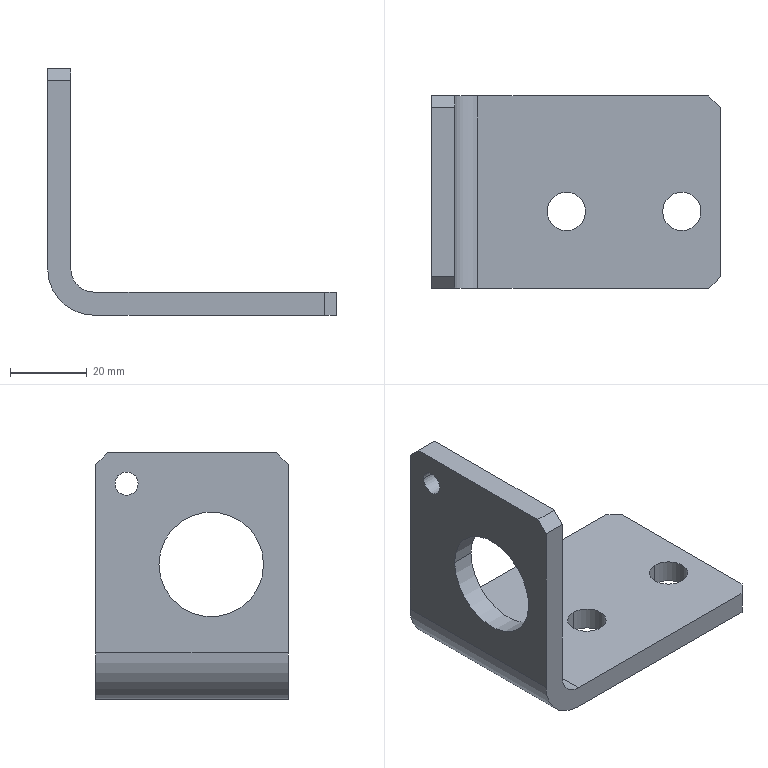Part | STEP file | [01]-14 | 1 solid | 22 faces | box 75 x 50 x 64 mm | volume 34035 mm3 | plane 12 | cylinder 10 | commonest cylinder face diameters 10 x4 6 x2 27.2 x2 12 x1 24 x1